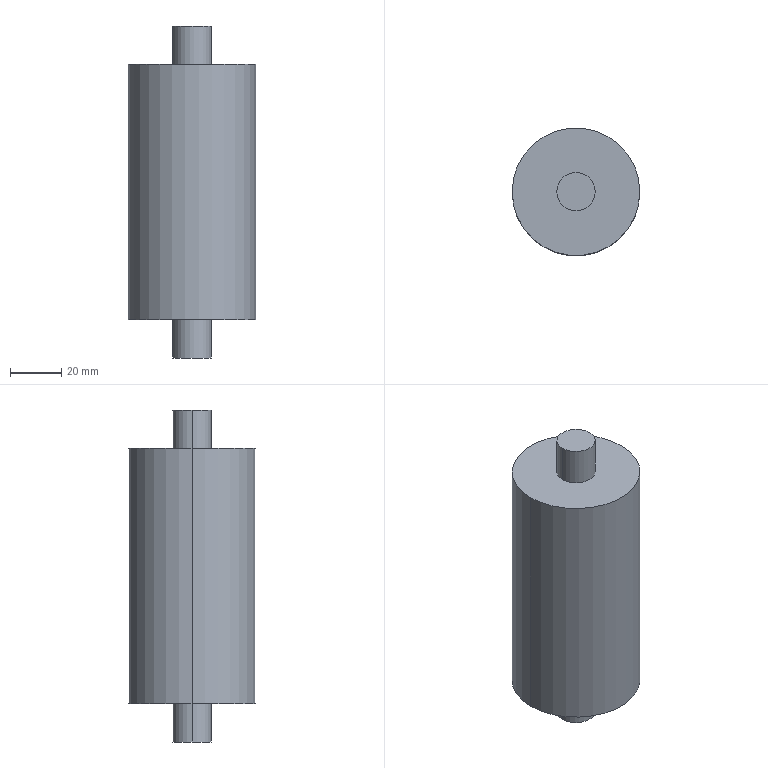Part | SolidWorks | features ICE 2, Extrusion 1 | 1 solid | 10 faces | box 50 x 50 x 130 mm | volume 201651 mm3 | cylinder 6 | plane 4 | commonest cylinder face diameters 15 x4 50 x2
STEP:
#1=CARTESIAN_POINT('',(-7.5,0.,-15.));
#2=VERTEX_POINT('',#1);
#3=CARTESIAN_POINT('',(7.5,0.,-15.));
#4=VERTEX_POINT('',#3);
#5=CARTESIAN_POINT('',(0.,0.,-15.));
#6=DIRECTION('',(0.,0.,-1.));
#7=DIRECTION('',(-1.,0.,0.));
#8=AXIS2_PLACEMENT_3D('',#5,#6,#7);
#9=CIRCLE('',#8,7.5);
#10=EDGE_CURVE('',#2,#4,#9,.T.);
#11=ORIENTED_EDGE('',*,*,#10,.F.);
#12=CARTESIAN_POINT('',(-7.5,0.,0.));
#13=VERTEX_POINT('',#12);
#14=CARTESIAN_POINT('',(-7.5,0.,-15.));
#15=DIRECTION('',(0.,0.,1.));
#16=VECTOR('',#15,1000.);
#17=LINE('',#14,#16);
#18=EDGE_CURVE('',#2,#13,#17,.T.);
#19=ORIENTED_EDGE('',*,*,#18,.T.);
#20=CARTESIAN_POINT('',(7.5,0.,0.));
#21=VERTEX_POINT('',#20);
#22=CARTESIAN_POINT('',(0.,0.,0.));
#23=DIRECTION('',(0.,0.,-1.));
#24=DIRECTION('',(-1.,0.,0.));
#25=AXIS2_PLACEMENT_3D('',#22,#23,#24);
#26=CIRCLE('',#25,7.5);
#27=EDGE_CURVE('',#13,#21,#26,.T.);
#28=ORIENTED_EDGE('',*,*,#27,.T.);
#29=CARTESIAN_POINT('',(7.5,0.,-15.));
#30=DIRECTION('',(0.,0.,1.));
#31=VECTOR('',#30,1000.);
#32=LINE('',#29,#31);
#33=EDGE_CURVE('',#4,#21,#32,.T.);
#34=ORIENTED_EDGE('',*,*,#33,.F.);
#35=EDGE_LOOP('',(#11,#19,#28,#34));
#36=FACE_OUTER_BOUND('',#35,.T.);
#37=CARTESIAN_POINT('',(0.,0.,-15.));
#38=DIRECTION('',(0.,0.,1.));
#39=DIRECTION('',(1.,0.,0.));
#40=AXIS2_PLACEMENT_3D('',#37,#38,#39);
#41=CYLINDRICAL_SURFACE('',#40,7.5);
#42=ADVANCED_FACE('',(#36),#41,.T.);
#43=CARTESIAN_POINT('',(7.5,0.,115.));
#44=VERTEX_POINT('',#43);
#45=CARTESIAN_POINT('',(-7.5,0.,115.));
#46=VERTEX_POINT('',#45);
#47=CARTESIAN_POINT('',(0.,0.,115.));
#48=DIRECTION('',(0.,0.,1.));
#49=DIRECTION('',(1.,0.,0.));
#50=AXIS2_PLACEMENT_3D('',#47,#48,#49);
#51=CIRCLE('',#50,7.5);
#52=EDGE_CURVE('',#44,#46,#51,.T.);
#53=ORIENTED_EDGE('',*,*,#52,.F.);
#54=CARTESIAN_POINT('',(7.5,0.,100.));
#55=VERTEX_POINT('',#54);
#56=CARTESIAN_POINT('',(7.5,0.,115.));
#57=DIRECTION('',(0.,0.,-1.));
#58=VECTOR('',#57,1000.);
#59=LINE('',#56,#58);
#60=EDGE_CURVE('',#44,#55,#59,.T.);
#61=ORIENTED_EDGE('',*,*,#60,.T.);
#62=CARTESIAN_POINT('',(-7.5,0.,100.));
#63=VERTEX_POINT('',#62);
#64=CARTESIAN_POINT('',(0.,0.,100.));
#65=DIRECTION('',(0.,0.,1.));
#66=DIRECTION('',(1.,0.,0.));
#67=AXIS2_PLACEMENT_3D('',#64,#65,#66);
#68=CIRCLE('',#67,7.5);
#69=EDGE_CURVE('',#55,#63,#68,.T.);
#70=ORIENTED_EDGE('',*,*,#69,.T.);
#71=CARTESIAN_POINT('',(-7.5,0.,115.));
#72=DIRECTION('',(0.,0.,-1.));
#73=VECTOR('',#72,1000.);
#74=LINE('',#71,#73);
#75=EDGE_CURVE('',#46,#63,#74,.T.);
#76=ORIENTED_EDGE('',*,*,#75,.F.);
#77=EDGE_LOOP('',(#53,#61,#70,#76));
#78=FACE_OUTER_BOUND('',#77,.T.);
#79=CARTESIAN_POINT('',(0.,0.,115.));
#80=DIRECTION('',(0.,0.,-1.));
#81=DIRECTION('',(-1.,0.,0.));
#82=AXIS2_PLACEMENT_3D('',#79,#80,#81);
#83=CYLINDRICAL_SURFACE('',#82,7.5);
#84=ADVANCED_FACE('',(#78),#83,.T.);
#85=CARTESIAN_POINT('',(25.,0.,100.));
#86=VERTEX_POINT('',#85);
#87=CARTESIAN_POINT('',(-25.,0.,100.));
#88=VERTEX_POINT('',#87);
#89=CARTESIAN_POINT('',(0.,0.,100.));
#90=DIRECTION('',(0.,0.,1.));
#91=DIRECTION('',(1.,0.,0.));
#92=AXIS2_PLACEMENT_3D('',#89,#90,#91);
#93=CIRCLE('',#92,25.);
#94=EDGE_CURVE('',#86,#88,#93,.T.);
#95=ORIENTED_EDGE('',*,*,#94,.F.);
#96=CARTESIAN_POINT('',(25.,0.,0.));
#97=VERTEX_POINT('',#96);
#98=CARTESIAN_POINT('',(25.,0.,100.));
#99=DIRECTION('',(0.,0.,-1.));
#100=VECTOR('',#99,1000.);
#101=LINE('',#98,#100);
#102=EDGE_CURVE('',#86,#97,#101,.T.);
#103=ORIENTED_EDGE('',*,*,#102,.T.);
#104=CARTESIAN_POINT('',(-25.,0.,0.));
#105=VERTEX_POINT('',#104);
#106=CARTESIAN_POINT('',(0.,0.,0.));
#107=DIRECTION('',(0.,0.,1.));
#108=DIRECTION('',(1.,0.,0.));
#109=AXIS2_PLACEMENT_3D('',#106,#107,#108);
#110=CIRCLE('',#109,25.);
#111=EDGE_CURVE('',#97,#105,#110,.T.);
#112=ORIENTED_EDGE('',*,*,#111,.T.);
#113=CARTESIAN_POINT('',(-25.,0.,100.));
#114=DIRECTION('',(0.,0.,-1.));
#115=VECTOR('',#114,1000.);
#116=LINE('',#113,#115);
#117=EDGE_CURVE('',#88,#105,#116,.T.);
#118=ORIENTED_EDGE('',*,*,#117,.F.);
#119=EDGE_LOOP('',(#95,#103,#112,#118));
#120=FACE_OUTER_BOUND('',#119,.T.);
#121=CARTESIAN_POINT('',(0.,0.,100.));
#122=DIRECTION('',(0.,0.,-1.));
#123=DIRECTION('',(-1.,0.,0.));
#124=AXIS2_PLACEMENT_3D('',#121,#122,#123);
#125=CYLINDRICAL_SURFACE('',#124,25.);
#126=ADVANCED_FACE('',(#120),#125,.T.);
#127=ORIENTED_EDGE('',*,*,#102,.F.);
#128=CARTESIAN_POINT('',(0.,0.,100.));
#129=DIRECTION('',(0.,0.,1.));
#130=DIRECTION('',(1.,0.,0.));
#131=AXIS2_PLACEMENT_3D('',#128,#129,#130);
#132=CIRCLE('',#131,25.);
#133=EDGE_CURVE('',#88,#86,#132,.T.);
#134=ORIENTED_EDGE('',*,*,#133,.F.);
#135=ORIENTED_EDGE('',*,*,#117,.T.);
#136=CARTESIAN_POINT('',(0.,0.,0.));
#137=DIRECTION('',(0.,0.,1.));
#138=DIRECTION('',(1.,0.,0.));
#139=AXIS2_PLACEMENT_3D('',#136,#137,#138);
#140=CIRCLE('',#139,25.);
#141=EDGE_CURVE('',#105,#97,#140,.T.);
#142=ORIENTED_EDGE('',*,*,#141,.T.);
#143=EDGE_LOOP('',(#127,#134,#135,#142));
#144=FACE_OUTER_BOUND('',#143,.T.);
#145=CARTESIAN_POINT('',(0.,0.,100.));
#146=DIRECTION('',(0.,0.,-1.));
#147=DIRECTION('',(-1.,0.,0.));
#148=AXIS2_PLACEMENT_3D('',#145,#146,#147);
#149=CYLINDRICAL_SURFACE('',#148,25.);
#150=ADVANCED_FACE('',(#144),#149,.T.);
#151=CARTESIAN_POINT('',(0.,0.,100.));
#152=DIRECTION('',(0.,0.,1.));
#153=DIRECTION('',(1.,0.,0.));
#154=AXIS2_PLACEMENT_3D('',#151,#152,#153);
#155=CIRCLE('',#154,7.5);
#156=EDGE_CURVE('',#63,#55,#155,.T.);
#157=ORIENTED_EDGE('',*,*,#156,.F.);
#158=ORIENTED_EDGE('',*,*,#69,.F.);
#159=EDGE_LOOP('',(#157,#158));
#160=FACE_BOUND('',#159,.T.);
#161=ORIENTED_EDGE('',*,*,#133,.T.);
#162=ORIENTED_EDGE('',*,*,#94,.T.);
#163=EDGE_LOOP('',(#161,#162));
#164=FACE_OUTER_BOUND('',#163,.T.);
#165=CARTESIAN_POINT('',(0.,0.,100.));
#166=DIRECTION('',(0.,0.,1.));
#167=DIRECTION('',(1.,0.,0.));
#168=AXIS2_PLACEMENT_3D('',#165,#166,#167);
#169=PLANE('',#168);
#170=ADVANCED_FACE('',(#160,#164),#169,.T.);
#171=CARTESIAN_POINT('',(0.,0.,0.));
#172=DIRECTION('',(0.,0.,-1.));
#173=DIRECTION('',(-1.,0.,0.));
#174=AXIS2_PLACEMENT_3D('',#171,#172,#173);
#175=CIRCLE('',#174,7.5);
#176=EDGE_CURVE('',#21,#13,#175,.T.);
#177=ORIENTED_EDGE('',*,*,#176,.F.);
#178=ORIENTED_EDGE('',*,*,#27,.F.);
#179=EDGE_LOOP('',(#177,#178));
#180=FACE_BOUND('',#179,.T.);
#181=ORIENTED_EDGE('',*,*,#141,.F.);
#182=ORIENTED_EDGE('',*,*,#111,.F.);
#183=EDGE_LOOP('',(#181,#182));
#184=FACE_OUTER_BOUND('',#183,.T.);
#185=CARTESIAN_POINT('',(0.,0.,0.));
#186=DIRECTION('',(0.,0.,1.));
#187=DIRECTION('',(1.,0.,0.));
#188=AXIS2_PLACEMENT_3D('',#185,#186,#187);
#189=PLANE('',#188);
#190=ADVANCED_FACE('',(#180,#184),#189,.F.);
#191=ORIENTED_EDGE('',*,*,#60,.F.);
#192=CARTESIAN_POINT('',(0.,0.,115.));
#193=DIRECTION('',(0.,0.,1.));
#194=DIRECTION('',(1.,0.,0.));
#195=AXIS2_PLACEMENT_3D('',#192,#193,#194);
#196=CIRCLE('',#195,7.5);
#197=EDGE_CURVE('',#46,#44,#196,.T.);
#198=ORIENTED_EDGE('',*,*,#197,.F.);
#199=ORIENTED_EDGE('',*,*,#75,.T.);
#200=ORIENTED_EDGE('',*,*,#156,.T.);
#201=EDGE_LOOP('',(#191,#198,#199,#200));
#202=FACE_OUTER_BOUND('',#201,.T.);
#203=CARTESIAN_POINT('',(0.,0.,115.));
#204=DIRECTION('',(0.,0.,-1.));
#205=DIRECTION('',(-1.,0.,0.));
#206=AXIS2_PLACEMENT_3D('',#203,#204,#205);
#207=CYLINDRICAL_SURFACE('',#206,7.5);
#208=ADVANCED_FACE('',(#202),#207,.T.);
#209=ORIENTED_EDGE('',*,*,#197,.T.);
#210=ORIENTED_EDGE('',*,*,#52,.T.);
#211=EDGE_LOOP('',(#209,#210));
#212=FACE_OUTER_BOUND('',#211,.T.);
#213=CARTESIAN_POINT('',(0.,0.,115.));
#214=DIRECTION('',(0.,0.,1.));
#215=DIRECTION('',(1.,0.,0.));
#216=AXIS2_PLACEMENT_3D('',#213,#214,#215);
#217=PLANE('',#216);
#218=ADVANCED_FACE('',(#212),#217,.T.);
#219=ORIENTED_EDGE('',*,*,#18,.F.);
#220=CARTESIAN_POINT('',(0.,0.,-15.));
#221=DIRECTION('',(0.,0.,-1.));
#222=DIRECTION('',(-1.,0.,0.));
#223=AXIS2_PLACEMENT_3D('',#220,#221,#222);
#224=CIRCLE('',#223,7.5);
#225=EDGE_CURVE('',#4,#2,#224,.T.);
#226=ORIENTED_EDGE('',*,*,#225,.F.);
#227=ORIENTED_EDGE('',*,*,#33,.T.);
#228=ORIENTED_EDGE('',*,*,#176,.T.);
#229=EDGE_LOOP('',(#219,#226,#227,#228));
#230=FACE_OUTER_BOUND('',#229,.T.);
#231=CARTESIAN_POINT('',(0.,0.,-15.));
#232=DIRECTION('',(0.,0.,1.));
#233=DIRECTION('',(1.,0.,0.));
#234=AXIS2_PLACEMENT_3D('',#231,#232,#233);
#235=CYLINDRICAL_SURFACE('',#234,7.5);
#236=ADVANCED_FACE('',(#230),#235,.T.);
#237=ORIENTED_EDGE('',*,*,#225,.T.);
#238=ORIENTED_EDGE('',*,*,#10,.T.);
#239=EDGE_LOOP('',(#237,#238));
#240=FACE_OUTER_BOUND('',#239,.T.);
#241=CARTESIAN_POINT('',(0.,0.,-15.));
#242=DIRECTION('',(0.,0.,-1.));
#243=DIRECTION('',(-1.,0.,0.));
#244=AXIS2_PLACEMENT_3D('',#241,#242,#243);
#245=PLANE('',#244);
#246=ADVANCED_FACE('',(#240),#245,.T.);
#247=CLOSED_SHELL('',(#42,#84,#126,#150,#170,#190,#208,#218,#236,#246));
#248=MANIFOLD_SOLID_BREP('',#247);
#249=CARTESIAN_POINT('',(0.,0.,0.));
#250=DIRECTION('',(0.,0.,1.));
#251=DIRECTION('',(1.,0.,0.));
#252=AXIS2_PLACEMENT_3D('',#249,#250,#251);
#253=(LENGTH_UNIT()NAMED_UNIT(*)SI_UNIT(.MILLI.,.METRE.));
#254=UNCERTAINTY_MEASURE_WITH_UNIT(LENGTH_MEASURE(0.00001),#253,'','');
#255=(NAMED_UNIT(*)PLANE_ANGLE_UNIT()SI_UNIT($,.RADIAN.));
#256=(NAMED_UNIT(*)SI_UNIT($,.STERADIAN.)SOLID_ANGLE_UNIT());
#257=(GEOMETRIC_REPRESENTATION_CONTEXT(3)GLOBAL_UNCERTAINTY_ASSIGNED_CONTEXT((#254))GLOBAL_UNIT_ASSIGNED_CONTEXT((#253,#255,#256))REPRESENTATION_CONTEXT('',''));
#258=ADVANCED_BREP_SHAPE_REPRESENTATION('',(#248,#252),#257);